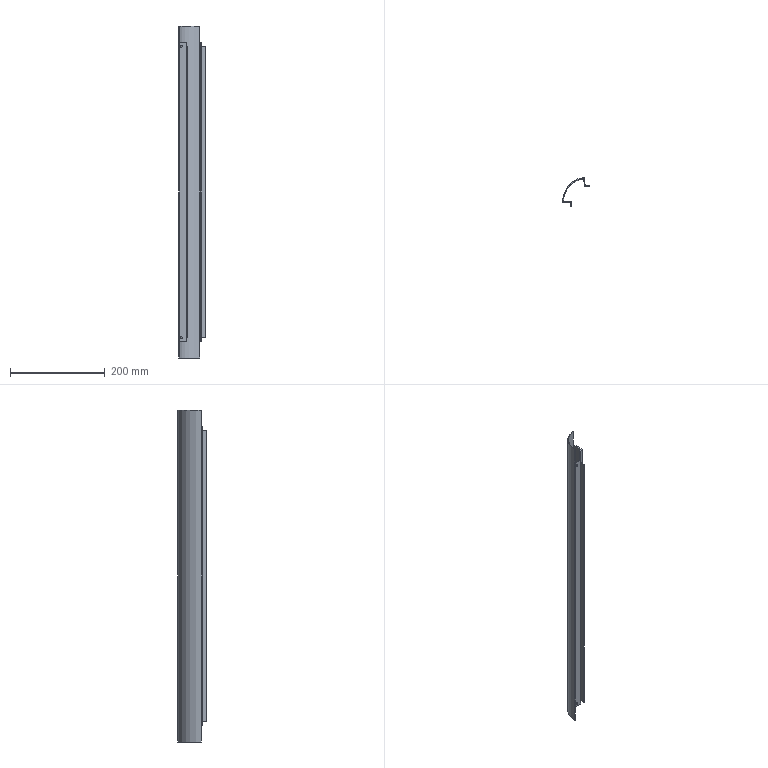Part | SolidWorks | features EdgeFlange 4, ICE 2, FlatPattern 1, SMBaseFlange 1, SheetMetal 1 | 1 solid | 51 faces | box 56.016 x 59.625 x 700 mm | volume 123971 mm3 | plane 36 | cylinder 15 | commonest cylinder face diameters 3 x5 4.5 x4 6.5 x4 97 x1 100 x1
STEP:
#1=CARTESIAN_POINT('',(-4.744,37.955,-175.));
#2=VERTEX_POINT('',#1);
#3=CARTESIAN_POINT('',(-5.551,44.404,-175.));
#4=VERTEX_POINT('',#3);
#5=CARTESIAN_POINT('',(-5.147,41.18,-175.));
#6=DIRECTION('',(0.9923,0.124,0.));
#7=DIRECTION('',(-0.124,0.9923,0.));
#8=AXIS2_PLACEMENT_3D('',#5,#6,#7);
#9=CIRCLE('',#8,3.25);
#10=EDGE_CURVE('',#2,#4,#9,.T.);
#11=ORIENTED_EDGE('',*,*,#10,.F.);
#12=CARTESIAN_POINT('',(-3.256,38.141,-175.));
#13=VERTEX_POINT('',#12);
#14=CARTESIAN_POINT('',(-4.744,37.955,-175.));
#15=DIRECTION('',(0.9923,0.124,0.));
#16=VECTOR('',#15,1000.);
#17=LINE('',#14,#16);
#18=EDGE_CURVE('',#2,#13,#17,.T.);
#19=ORIENTED_EDGE('',*,*,#18,.T.);
#20=CARTESIAN_POINT('',(-4.062,44.59,-175.));
#21=VERTEX_POINT('',#20);
#22=CARTESIAN_POINT('',(-3.659,41.366,-175.));
#23=DIRECTION('',(0.9923,0.124,0.));
#24=DIRECTION('',(-0.124,0.9923,0.));
#25=AXIS2_PLACEMENT_3D('',#22,#23,#24);
#26=CIRCLE('',#25,3.25);
#27=EDGE_CURVE('',#13,#21,#26,.T.);
#28=ORIENTED_EDGE('',*,*,#27,.T.);
#29=CARTESIAN_POINT('',(-5.551,44.404,-175.));
#30=DIRECTION('',(0.9923,0.124,0.));
#31=VECTOR('',#30,1000.);
#32=LINE('',#29,#31);
#33=EDGE_CURVE('',#4,#21,#32,.T.);
#34=ORIENTED_EDGE('',*,*,#33,.F.);
#35=EDGE_LOOP('',(#11,#19,#28,#34));
#36=FACE_OUTER_BOUND('',#35,.T.);
#37=CARTESIAN_POINT('',(-5.147,41.18,-175.));
#38=DIRECTION('',(0.9923,0.124,0.));
#39=DIRECTION('',(-0.124,0.9923,0.));
#40=AXIS2_PLACEMENT_3D('',#37,#38,#39);
#41=CYLINDRICAL_SURFACE('',#40,3.25);
#42=ADVANCED_FACE('',(#36),#41,.F.);
#43=CARTESIAN_POINT('',(-4.744,37.955,175.));
#44=VERTEX_POINT('',#43);
#45=CARTESIAN_POINT('',(-5.551,44.404,175.));
#46=VERTEX_POINT('',#45);
#47=CARTESIAN_POINT('',(-5.147,41.18,175.));
#48=DIRECTION('',(0.9923,0.124,0.));
#49=DIRECTION('',(-0.124,0.9923,0.));
#50=AXIS2_PLACEMENT_3D('',#47,#48,#49);
#51=CIRCLE('',#50,3.25);
#52=EDGE_CURVE('',#44,#46,#51,.T.);
#53=ORIENTED_EDGE('',*,*,#52,.F.);
#54=CARTESIAN_POINT('',(-3.256,38.141,175.));
#55=VERTEX_POINT('',#54);
#56=CARTESIAN_POINT('',(-4.744,37.955,175.));
#57=DIRECTION('',(0.9923,0.124,0.));
#58=VECTOR('',#57,1000.);
#59=LINE('',#56,#58);
#60=EDGE_CURVE('',#44,#55,#59,.T.);
#61=ORIENTED_EDGE('',*,*,#60,.T.);
#62=CARTESIAN_POINT('',(-4.062,44.59,175.));
#63=VERTEX_POINT('',#62);
#64=CARTESIAN_POINT('',(-3.659,41.366,175.));
#65=DIRECTION('',(0.9923,0.124,0.));
#66=DIRECTION('',(-0.124,0.9923,0.));
#67=AXIS2_PLACEMENT_3D('',#64,#65,#66);
#68=CIRCLE('',#67,3.25);
#69=EDGE_CURVE('',#55,#63,#68,.T.);
#70=ORIENTED_EDGE('',*,*,#69,.T.);
#71=CARTESIAN_POINT('',(-5.551,44.404,175.));
#72=DIRECTION('',(0.9923,0.124,0.));
#73=VECTOR('',#72,1000.);
#74=LINE('',#71,#73);
#75=EDGE_CURVE('',#46,#63,#74,.T.);
#76=ORIENTED_EDGE('',*,*,#75,.F.);
#77=EDGE_LOOP('',(#53,#61,#70,#76));
#78=FACE_OUTER_BOUND('',#77,.T.);
#79=CARTESIAN_POINT('',(-5.147,41.18,175.));
#80=DIRECTION('',(0.9923,0.124,0.));
#81=DIRECTION('',(-0.124,0.9923,0.));
#82=AXIS2_PLACEMENT_3D('',#79,#80,#81);
#83=CYLINDRICAL_SURFACE('',#82,3.25);
#84=ADVANCED_FACE('',(#78),#83,.F.);
#85=CARTESIAN_POINT('',(-46.75,0.,-307.5));
#86=VERTEX_POINT('',#85);
#87=CARTESIAN_POINT('',(-42.25,0.,-307.5));
#88=VERTEX_POINT('',#87);
#89=CARTESIAN_POINT('',(-44.5,0.,-307.5));
#90=DIRECTION('',(0.,-1.,0.));
#91=DIRECTION('',(1.,0.,0.));
#92=AXIS2_PLACEMENT_3D('',#89,#90,#91);
#93=CIRCLE('',#92,2.25);
#94=EDGE_CURVE('',#86,#88,#93,.T.);
#95=ORIENTED_EDGE('',*,*,#94,.F.);
#96=CARTESIAN_POINT('',(-46.75,-1.5,-307.5));
#97=VERTEX_POINT('',#96);
#98=CARTESIAN_POINT('',(-46.75,0.,-307.5));
#99=DIRECTION('',(0.,-1.,0.));
#100=VECTOR('',#99,1000.);
#101=LINE('',#98,#100);
#102=EDGE_CURVE('',#86,#97,#101,.T.);
#103=ORIENTED_EDGE('',*,*,#102,.T.);
#104=CARTESIAN_POINT('',(-42.25,-1.5,-307.5));
#105=VERTEX_POINT('',#104);
#106=CARTESIAN_POINT('',(-44.5,-1.5,-307.5));
#107=DIRECTION('',(0.,-1.,0.));
#108=DIRECTION('',(1.,0.,0.));
#109=AXIS2_PLACEMENT_3D('',#106,#107,#108);
#110=CIRCLE('',#109,2.25);
#111=EDGE_CURVE('',#97,#105,#110,.T.);
#112=ORIENTED_EDGE('',*,*,#111,.T.);
#113=CARTESIAN_POINT('',(-42.25,0.,-307.5));
#114=DIRECTION('',(0.,-1.,0.));
#115=VECTOR('',#114,1000.);
#116=LINE('',#113,#115);
#117=EDGE_CURVE('',#88,#105,#116,.T.);
#118=ORIENTED_EDGE('',*,*,#117,.F.);
#119=EDGE_LOOP('',(#95,#103,#112,#118));
#120=FACE_OUTER_BOUND('',#119,.T.);
#121=CARTESIAN_POINT('',(-44.5,0.,-307.5));
#122=DIRECTION('',(0.,-1.,0.));
#123=DIRECTION('',(1.,0.,0.));
#124=AXIS2_PLACEMENT_3D('',#121,#122,#123);
#125=CYLINDRICAL_SURFACE('',#124,2.25);
#126=ADVANCED_FACE('',(#120),#125,.F.);
#127=CARTESIAN_POINT('',(-46.75,0.,307.5));
#128=VERTEX_POINT('',#127);
#129=CARTESIAN_POINT('',(-42.25,0.,307.5));
#130=VERTEX_POINT('',#129);
#131=CARTESIAN_POINT('',(-44.5,0.,307.5));
#132=DIRECTION('',(0.,-1.,0.));
#133=DIRECTION('',(1.,0.,0.));
#134=AXIS2_PLACEMENT_3D('',#131,#132,#133);
#135=CIRCLE('',#134,2.25);
#136=EDGE_CURVE('',#128,#130,#135,.T.);
#137=ORIENTED_EDGE('',*,*,#136,.F.);
#138=CARTESIAN_POINT('',(-46.75,-1.5,307.5));
#139=VERTEX_POINT('',#138);
#140=CARTESIAN_POINT('',(-46.75,0.,307.5));
#141=DIRECTION('',(0.,-1.,0.));
#142=VECTOR('',#141,1000.);
#143=LINE('',#140,#142);
#144=EDGE_CURVE('',#128,#139,#143,.T.);
#145=ORIENTED_EDGE('',*,*,#144,.T.);
#146=CARTESIAN_POINT('',(-42.25,-1.5,307.5));
#147=VERTEX_POINT('',#146);
#148=CARTESIAN_POINT('',(-44.5,-1.5,307.5));
#149=DIRECTION('',(0.,-1.,0.));
#150=DIRECTION('',(1.,0.,0.));
#151=AXIS2_PLACEMENT_3D('',#148,#149,#150);
#152=CIRCLE('',#151,2.25);
#153=EDGE_CURVE('',#139,#147,#152,.T.);
#154=ORIENTED_EDGE('',*,*,#153,.T.);
#155=CARTESIAN_POINT('',(-42.25,0.,307.5));
#156=DIRECTION('',(0.,-1.,0.));
#157=VECTOR('',#156,1000.);
#158=LINE('',#155,#157);
#159=EDGE_CURVE('',#130,#147,#158,.T.);
#160=ORIENTED_EDGE('',*,*,#159,.F.);
#161=EDGE_LOOP('',(#137,#145,#154,#160));
#162=FACE_OUTER_BOUND('',#161,.T.);
#163=CARTESIAN_POINT('',(-44.5,0.,307.5));
#164=DIRECTION('',(0.,-1.,0.));
#165=DIRECTION('',(1.,0.,0.));
#166=AXIS2_PLACEMENT_3D('',#163,#164,#165);
#167=CYLINDRICAL_SURFACE('',#166,2.25);
#168=ADVANCED_FACE('',(#162),#167,.F.);
#169=CARTESIAN_POINT('',(-6.202,49.614,315.));
#170=VERTEX_POINT('',#169);
#171=CARTESIAN_POINT('',(-6.016,49.625,315.));
#172=VERTEX_POINT('',#171);
#173=CARTESIAN_POINT('',(-6.016,48.125,315.));
#174=DIRECTION('',(0.,0.,-1.));
#175=DIRECTION('',(0.,1.,0.));
#176=AXIS2_PLACEMENT_3D('',#173,#174,#175);
#177=CIRCLE('',#176,1.5);
#178=EDGE_CURVE('',#170,#172,#177,.T.);
#179=ORIENTED_EDGE('',*,*,#178,.T.);
#180=CARTESIAN_POINT('',(-6.016,49.625,-315.));
#181=VERTEX_POINT('',#180);
#182=CARTESIAN_POINT('',(-6.016,49.625,-315.));
#183=DIRECTION('',(0.,0.,-1.));
#184=VECTOR('',#183,1000.);
#185=LINE('',#182,#184);
#186=EDGE_CURVE('',#172,#181,#185,.T.);
#187=ORIENTED_EDGE('',*,*,#186,.T.);
#188=CARTESIAN_POINT('',(-6.202,49.614,-315.));
#189=VERTEX_POINT('',#188);
#190=CARTESIAN_POINT('',(-6.016,48.125,-315.));
#191=DIRECTION('',(0.,0.,-1.));
#192=DIRECTION('',(0.,1.,0.));
#193=AXIS2_PLACEMENT_3D('',#190,#191,#192);
#194=CIRCLE('',#193,1.5);
#195=EDGE_CURVE('',#189,#181,#194,.T.);
#196=ORIENTED_EDGE('',*,*,#195,.F.);
#197=CARTESIAN_POINT('',(-6.202,49.614,-315.));
#198=DIRECTION('',(0.,0.,-1.));
#199=VECTOR('',#198,1000.);
#200=LINE('',#197,#199);
#201=EDGE_CURVE('',#170,#189,#200,.T.);
#202=ORIENTED_EDGE('',*,*,#201,.F.);
#203=EDGE_LOOP('',(#179,#187,#196,#202));
#204=FACE_OUTER_BOUND('',#203,.T.);
#205=CARTESIAN_POINT('',(-6.016,48.125,-315.));
#206=DIRECTION('',(0.,0.,-1.));
#207=DIRECTION('',(0.,1.,0.));
#208=AXIS2_PLACEMENT_3D('',#205,#206,#207);
#209=CYLINDRICAL_SURFACE('',#208,1.5);
#210=ADVANCED_FACE('',(#204),#209,.T.);
#211=CARTESIAN_POINT('',(-33.,0.,306.5));
#212=VERTEX_POINT('',#211);
#213=CARTESIAN_POINT('',(-33.,-1.5,306.5));
#214=VERTEX_POINT('',#213);
#215=CARTESIAN_POINT('',(-33.,0.,306.5));
#216=DIRECTION('',(0.,-1.,0.));
#217=VECTOR('',#216,1000.);
#218=LINE('',#215,#217);
#219=EDGE_CURVE('',#212,#214,#218,.T.);
#220=ORIENTED_EDGE('',*,*,#219,.F.);
#221=CARTESIAN_POINT('',(-33.,0.,315.));
#222=VERTEX_POINT('',#221);
#223=CARTESIAN_POINT('',(-33.,0.,315.));
#224=DIRECTION('',(0.,0.,1.));
#225=VECTOR('',#224,1000.);
#226=LINE('',#223,#225);
#227=EDGE_CURVE('',#212,#222,#226,.T.);
#228=ORIENTED_EDGE('',*,*,#227,.T.);
#229=CARTESIAN_POINT('',(-33.,-1.5,315.));
#230=VERTEX_POINT('',#229);
#231=CARTESIAN_POINT('',(-33.,-1.5,315.));
#232=DIRECTION('',(0.,1.,0.));
#233=VECTOR('',#232,1000.);
#234=LINE('',#231,#233);
#235=EDGE_CURVE('',#230,#222,#234,.T.);
#236=ORIENTED_EDGE('',*,*,#235,.F.);
#237=CARTESIAN_POINT('',(-33.,-1.5,315.));
#238=DIRECTION('',(0.,0.,1.));
#239=VECTOR('',#238,1000.);
#240=LINE('',#237,#239);
#241=EDGE_CURVE('',#214,#230,#240,.T.);
#242=ORIENTED_EDGE('',*,*,#241,.F.);
#243=EDGE_LOOP('',(#220,#228,#236,#242));
#244=FACE_OUTER_BOUND('',#243,.T.);
#245=CARTESIAN_POINT('',(-33.,-1.5,315.));
#246=DIRECTION('',(-1.,0.,0.));
#247=DIRECTION('',(0.,-1.,0.));
#248=AXIS2_PLACEMENT_3D('',#245,#246,#247);
#249=PLANE('',#248);
#250=ADVANCED_FACE('',(#244),#249,.F.);
#251=CARTESIAN_POINT('',(-50.,0.,350.));
#252=VERTEX_POINT('',#251);
#253=CARTESIAN_POINT('',(-50.,0.,315.));
#254=VERTEX_POINT('',#253);
#255=CARTESIAN_POINT('',(-50.,0.,350.));
#256=DIRECTION('',(0.,0.,-1.));
#257=VECTOR('',#256,1000.);
#258=LINE('',#255,#257);
#259=EDGE_CURVE('',#252,#254,#258,.T.);
#260=ORIENTED_EDGE('',*,*,#259,.T.);
#261=CARTESIAN_POINT('',(-48.5,0.,315.));
#262=VERTEX_POINT('',#261);
#263=CARTESIAN_POINT('',(-50.,0.,315.));
#264=DIRECTION('',(1.,0.,0.));
#265=VECTOR('',#264,1000.);
#266=LINE('',#263,#265);
#267=EDGE_CURVE('',#254,#262,#266,.T.);
#268=ORIENTED_EDGE('',*,*,#267,.T.);
#269=CARTESIAN_POINT('',(-48.5,0.,350.));
#270=VERTEX_POINT('',#269);
#271=CARTESIAN_POINT('',(-48.5,0.,350.));
#272=DIRECTION('',(0.,0.,-1.));
#273=VECTOR('',#272,1000.);
#274=LINE('',#271,#273);
#275=EDGE_CURVE('',#270,#262,#274,.T.);
#276=ORIENTED_EDGE('',*,*,#275,.F.);
#277=CARTESIAN_POINT('',(-48.5,0.,350.));
#278=DIRECTION('',(-1.,0.,0.));
#279=VECTOR('',#278,1000.);
#280=LINE('',#277,#279);
#281=EDGE_CURVE('',#270,#252,#280,.T.);
#282=ORIENTED_EDGE('',*,*,#281,.T.);
#283=EDGE_LOOP('',(#260,#268,#276,#282));
#284=FACE_OUTER_BOUND('',#283,.T.);
#285=CARTESIAN_POINT('',(-48.5,0.,350.));
#286=DIRECTION('',(0.,-1.,0.));
#287=DIRECTION('',(1.,0.,0.));
#288=AXIS2_PLACEMENT_3D('',#285,#286,#287);
#289=PLANE('',#288);
#290=ADVANCED_FACE('',(#284),#289,.T.);
#291=CARTESIAN_POINT('',(-4.093,32.745,306.5));
#292=VERTEX_POINT('',#291);
#293=CARTESIAN_POINT('',(-4.093,32.745,315.));
#294=VERTEX_POINT('',#293);
#295=CARTESIAN_POINT('',(-4.093,32.745,315.));
#296=DIRECTION('',(0.,0.,1.));
#297=VECTOR('',#296,1000.);
#298=LINE('',#295,#297);
#299=EDGE_CURVE('',#292,#294,#298,.T.);
#300=ORIENTED_EDGE('',*,*,#299,.F.);
#301=CARTESIAN_POINT('',(-2.605,32.931,306.5));
#302=VERTEX_POINT('',#301);
#303=CARTESIAN_POINT('',(-4.093,32.745,306.5));
#304=DIRECTION('',(0.9923,0.124,0.));
#305=VECTOR('',#304,1000.);
#306=LINE('',#303,#305);
#307=EDGE_CURVE('',#292,#302,#306,.T.);
#308=ORIENTED_EDGE('',*,*,#307,.T.);
#309=CARTESIAN_POINT('',(-2.605,32.931,315.));
#310=VERTEX_POINT('',#309);
#311=CARTESIAN_POINT('',(-2.605,32.931,315.));
#312=DIRECTION('',(0.,0.,1.));
#313=VECTOR('',#312,1000.);
#314=LINE('',#311,#313);
#315=EDGE_CURVE('',#302,#310,#314,.T.);
#316=ORIENTED_EDGE('',*,*,#315,.T.);
#317=CARTESIAN_POINT('',(-2.605,32.931,315.));
#318=DIRECTION('',(-0.9923,-0.124,0.));
#319=VECTOR('',#318,1000.);
#320=LINE('',#317,#319);
#321=EDGE_CURVE('',#310,#294,#320,.T.);
#322=ORIENTED_EDGE('',*,*,#321,.T.);
#323=EDGE_LOOP('',(#300,#308,#316,#322));
#324=FACE_OUTER_BOUND('',#323,.T.);
#325=CARTESIAN_POINT('',(-2.605,32.931,315.));
#326=DIRECTION('',(0.124,-0.9923,0.));
#327=DIRECTION('',(0.9923,0.124,0.));
#328=AXIS2_PLACEMENT_3D('',#325,#326,#327);
#329=PLANE('',#328);
#330=ADVANCED_FACE('',(#324),#329,.T.);
#331=CARTESIAN_POINT('',(-6.202,49.614,-350.));
#332=VERTEX_POINT('',#331);
#333=CARTESIAN_POINT('',(-6.202,49.614,350.));
#334=DIRECTION('',(0.,0.,-1.));
#335=VECTOR('',#334,1000.);
#336=LINE('',#333,#335);
#337=EDGE_CURVE('',#189,#332,#336,.T.);
#338=ORIENTED_EDGE('',*,*,#337,.F.);
#339=CARTESIAN_POINT('',(-6.016,48.125,-315.));
#340=VERTEX_POINT('',#339);
#341=CARTESIAN_POINT('',(-6.202,49.614,-315.));
#342=DIRECTION('',(0.124,-0.9923,0.));
#343=VECTOR('',#342,1000.);
#344=LINE('',#341,#343);
#345=EDGE_CURVE('',#189,#340,#344,.T.);
#346=ORIENTED_EDGE('',*,*,#345,.T.);
#347=CARTESIAN_POINT('',(-6.016,48.125,-350.));
#348=VERTEX_POINT('',#347);
#349=CARTESIAN_POINT('',(-6.016,48.125,350.));
#350=DIRECTION('',(0.,0.,-1.));
#351=VECTOR('',#350,1000.);
#352=LINE('',#349,#351);
#353=EDGE_CURVE('',#340,#348,#352,.T.);
#354=ORIENTED_EDGE('',*,*,#353,.T.);
#355=CARTESIAN_POINT('',(-6.202,49.614,-350.));
#356=DIRECTION('',(0.124,-0.9923,0.));
#357=VECTOR('',#356,1000.);
#358=LINE('',#355,#357);
#359=EDGE_CURVE('',#332,#348,#358,.T.);
#360=ORIENTED_EDGE('',*,*,#359,.F.);
#361=EDGE_LOOP('',(#338,#346,#354,#360));
#362=FACE_OUTER_BOUND('',#361,.T.);
#363=CARTESIAN_POINT('',(-6.202,49.614,350.));
#364=DIRECTION('',(0.9923,0.124,0.));
#365=DIRECTION('',(-0.124,0.9923,0.));
#366=AXIS2_PLACEMENT_3D('',#363,#364,#365);
#367=PLANE('',#366);
#368=ADVANCED_FACE('',(#362),#367,.T.);
#369=CARTESIAN_POINT('',(-50.,0.,-350.));
#370=VERTEX_POINT('',#369);
#371=CARTESIAN_POINT('',(0.,0.,-350.));
#372=DIRECTION('',(0.,0.,1.));
#373=DIRECTION('',(1.,0.,0.));
#374=AXIS2_PLACEMENT_3D('',#371,#372,#373);
#375=CIRCLE('',#374,50.);
#376=EDGE_CURVE('',#332,#370,#375,.T.);
#377=ORIENTED_EDGE('',*,*,#376,.T.);
#378=CARTESIAN_POINT('',(-50.,0.,-315.));
#379=VERTEX_POINT('',#378);
#380=CARTESIAN_POINT('',(-50.,0.,350.));
#381=DIRECTION('',(0.,0.,-1.));
#382=VECTOR('',#381,1000.);
#383=LINE('',#380,#382);
#384=EDGE_CURVE('',#379,#370,#383,.T.);
#385=ORIENTED_EDGE('',*,*,#384,.F.);
#386=CARTESIAN_POINT('',(-50.,0.,315.));
#387=DIRECTION('',(0.,0.,-1.));
#388=VECTOR('',#387,1000.);
#389=LINE('',#386,#388);
#390=EDGE_CURVE('',#254,#379,#389,.T.);
#391=ORIENTED_EDGE('',*,*,#390,.F.);
#392=ORIENTED_EDGE('',*,*,#259,.F.);
#393=CARTESIAN_POINT('',(-6.202,49.614,350.));
#394=VERTEX_POINT('',#393);
#395=CARTESIAN_POINT('',(0.,0.,350.));
#396=DIRECTION('',(0.,0.,1.));
#397=DIRECTION('',(1.,0.,0.));
#398=AXIS2_PLACEMENT_3D('',#395,#396,#397);
#399=CIRCLE('',#398,50.);
#400=EDGE_CURVE('',#394,#252,#399,.T.);
#401=ORIENTED_EDGE('',*,*,#400,.F.);
#402=CARTESIAN_POINT('',(-6.202,49.614,350.));
#403=DIRECTION('',(0.,0.,-1.));
#404=VECTOR('',#403,1000.);
#405=LINE('',#402,#404);
#406=EDGE_CURVE('',#394,#170,#405,.T.);
#407=ORIENTED_EDGE('',*,*,#406,.T.);
#408=ORIENTED_EDGE('',*,*,#201,.T.);
#409=ORIENTED_EDGE('',*,*,#337,.T.);
#410=EDGE_LOOP('',(#377,#385,#391,#392,#401,#407,#408,#409));
#411=FACE_OUTER_BOUND('',#410,.T.);
#412=CARTESIAN_POINT('',(0.,0.,350.));
#413=DIRECTION('',(0.,0.,-1.));
#414=DIRECTION('',(-1.,0.,0.));
#415=AXIS2_PLACEMENT_3D('',#412,#413,#414);
#416=CYLINDRICAL_SURFACE('',#415,50.);
#417=ADVANCED_FACE('',(#411),#416,.T.);
#418=CARTESIAN_POINT('',(-48.5,0.,-315.));
#419=VERTEX_POINT('',#418);
#420=CARTESIAN_POINT('',(-50.,0.,-315.));
#421=DIRECTION('',(1.,0.,0.));
#422=VECTOR('',#421,1000.);
#423=LINE('',#420,#422);
#424=EDGE_CURVE('',#379,#419,#423,.T.);
#425=ORIENTED_EDGE('',*,*,#424,.F.);
#426=ORIENTED_EDGE('',*,*,#384,.T.);
#427=CARTESIAN_POINT('',(-48.5,0.,-350.));
#428=VERTEX_POINT('',#427);
#429=CARTESIAN_POINT('',(-48.5,0.,-350.));
#430=DIRECTION('',(-1.,0.,0.));
#431=VECTOR('',#430,1000.);
#432=LINE('',#429,#431);
#433=EDGE_CURVE('',#428,#370,#432,.T.);
#434=ORIENTED_EDGE('',*,*,#433,.F.);
#435=CARTESIAN_POINT('',(-48.5,0.,350.));
#436=DIRECTION('',(0.,0.,-1.));
#437=VECTOR('',#436,1000.);
#438=LINE('',#435,#437);
#439=EDGE_CURVE('',#419,#428,#438,.T.);
#440=ORIENTED_EDGE('',*,*,#439,.F.);
#441=EDGE_LOOP('',(#425,#426,#434,#440));
#442=FACE_OUTER_BOUND('',#441,.T.);
#443=CARTESIAN_POINT('',(-48.5,0.,350.));
#444=DIRECTION('',(0.,-1.,0.));
#445=DIRECTION('',(1.,0.,0.));
#446=AXIS2_PLACEMENT_3D('',#443,#444,#445);
#447=PLANE('',#446);
#448=ADVANCED_FACE('',(#442),#447,.T.);
#449=CARTESIAN_POINT('',(0.,0.,-350.));
#450=DIRECTION('',(0.,0.,1.));
#451=DIRECTION('',(1.,0.,0.));
#452=AXIS2_PLACEMENT_3D('',#449,#450,#451);
#453=CIRCLE('',#452,48.5);
#454=EDGE_CURVE('',#348,#428,#453,.T.);
#455=ORIENTED_EDGE('',*,*,#454,.F.);
#456=ORIENTED_EDGE('',*,*,#353,.F.);
#457=CARTESIAN_POINT('',(-6.016,48.125,315.));
#458=VERTEX_POINT('',#457);
#459=CARTESIAN_POINT('',(-6.016,48.125,-315.));
#460=DIRECTION('',(0.,0.,-1.));
#461=VECTOR('',#460,1000.);
#462=LINE('',#459,#461);
#463=EDGE_CURVE('',#458,#340,#462,.T.);
#464=ORIENTED_EDGE('',*,*,#463,.F.);
#465=CARTESIAN_POINT('',(-6.016,48.125,350.));
#466=VERTEX_POINT('',#465);
#467=CARTESIAN_POINT('',(-6.016,48.125,350.));
#468=DIRECTION('',(0.,0.,-1.));
#469=VECTOR('',#468,1000.);
#470=LINE('',#467,#469);
#471=EDGE_CURVE('',#466,#458,#470,.T.);
#472=ORIENTED_EDGE('',*,*,#471,.F.);
#473=CARTESIAN_POINT('',(0.,0.,350.));
#474=DIRECTION('',(0.,0.,1.));
#475=DIRECTION('',(1.,0.,0.));
#476=AXIS2_PLACEMENT_3D('',#473,#474,#475);
#477=CIRCLE('',#476,48.5);
#478=EDGE_CURVE('',#466,#270,#477,.T.);
#479=ORIENTED_EDGE('',*,*,#478,.T.);
#480=ORIENTED_EDGE('',*,*,#275,.T.);
#481=CARTESIAN_POINT('',(-48.5,0.,315.));
#482=DIRECTION('',(0.,0.,-1.));
#483=VECTOR('',#482,1000.);
#484=LINE('',#481,#483);
#485=EDGE_CURVE('',#262,#419,#484,.T.);
#486=ORIENTED_EDGE('',*,*,#485,.T.);
#487=ORIENTED_EDGE('',*,*,#439,.T.);
#488=EDGE_LOOP('',(#455,#456,#464,#472,#479,#480,#486,#487));
#489=FACE_OUTER_BOUND('',#488,.T.);
#490=CARTESIAN_POINT('',(0.,0.,350.));
#491=DIRECTION('',(0.,0.,-1.));
#492=DIRECTION('',(-1.,0.,0.));
#493=AXIS2_PLACEMENT_3D('',#490,#491,#492);
#494=CYLINDRICAL_SURFACE('',#493,48.5);
#495=ADVANCED_FACE('',(#489),#494,.F.);
#496=CARTESIAN_POINT('',(-6.202,49.614,315.));
#497=DIRECTION('',(0.124,-0.9923,0.));
#498=VECTOR('',#497,1000.);
#499=LINE('',#496,#498);
#500=EDGE_CURVE('',#170,#458,#499,.T.);
#501=ORIENTED_EDGE('',*,*,#500,.F.);
#502=ORIENTED_EDGE('',*,*,#406,.F.);
#503=CARTESIAN_POINT('',(-6.202,49.614,350.));
#504=DIRECTION('',(0.124,-0.9923,0.));
#505=VECTOR('',#504,1000.);
#506=LINE('',#503,#505);
#507=EDGE_CURVE('',#394,#466,#506,.T.);
#508=ORIENTED_EDGE('',*,*,#507,.T.);
#509=ORIENTED_EDGE('',*,*,#471,.T.);
#510=EDGE_LOOP('',(#501,#502,#508,#509));
#511=FACE_OUTER_BOUND('',#510,.T.);
#512=CARTESIAN_POINT('',(-6.202,49.614,350.));
#513=DIRECTION('',(0.9923,0.124,0.));
#514=DIRECTION('',(-0.124,0.9923,0.));
#515=AXIS2_PLACEMENT_3D('',#512,#513,#514);
#516=PLANE('',#515);
#517=ADVANCED_FACE('',(#511),#516,.T.);
#518=ORIENTED_EDGE('',*,*,#400,.T.);
#519=ORIENTED_EDGE('',*,*,#281,.F.);
#520=ORIENTED_EDGE('',*,*,#478,.F.);
#521=ORIENTED_EDGE('',*,*,#507,.F.);
#522=EDGE_LOOP('',(#518,#519,#520,#521));
#523=FACE_OUTER_BOUND('',#522,.T.);
#524=CARTESIAN_POINT('',(0.,0.,350.));
#525=DIRECTION('',(0.,0.,1.));
#526=DIRECTION('',(1.,0.,0.));
#527=AXIS2_PLACEMENT_3D('',#524,#525,#526);
#528=PLANE('',#527);
#529=ADVANCED_FACE('',(#523),#528,.T.);
#530=ORIENTED_EDGE('',*,*,#376,.F.);
#531=ORIENTED_EDGE('',*,*,#359,.T.);
#532=ORIENTED_EDGE('',*,*,#454,.T.);
#533=ORIENTED_EDGE('',*,*,#433,.T.);
#534=EDGE_LOOP('',(#530,#531,#532,#533));
#535=FACE_OUTER_BOUND('',#534,.T.);
#536=CARTESIAN_POINT('',(0.,0.,-350.));
#537=DIRECTION('',(0.,0.,1.));
#538=DIRECTION('',(1.,0.,0.));
#539=AXIS2_PLACEMENT_3D('',#536,#537,#538);
#540=PLANE('',#539);
#541=ADVANCED_FACE('',(#535),#540,.F.);
#542=ORIENTED_EDGE('',*,*,#178,.F.);
#543=ORIENTED_EDGE('',*,*,#500,.T.);
#544=CARTESIAN_POINT('',(-4.527,48.312,315.));
#545=VERTEX_POINT('',#544);
#546=CARTESIAN_POINT('',(-4.527,48.312,315.));
#547=DIRECTION('',(-0.9923,-0.124,0.));
#548=VECTOR('',#547,1000.);
#549=LINE('',#546,#548);
#550=EDGE_CURVE('',#545,#458,#549,.T.);
#551=ORIENTED_EDGE('',*,*,#550,.F.);
#552=CARTESIAN_POINT('',(-6.016,48.125,315.));
#553=DIRECTION('',(0.,0.,-1.));
#554=DIRECTION('',(0.,1.,0.));
#555=AXIS2_PLACEMENT_3D('',#552,#553,#554);
#556=CIRCLE('',#555,1.5);
#557=EDGE_CURVE('',#172,#545,#556,.T.);
#558=ORIENTED_EDGE('',*,*,#557,.F.);
#559=EDGE_LOOP('',(#542,#543,#551,#558));
#560=FACE_OUTER_BOUND('',#559,.T.);
#561=CARTESIAN_POINT('',(-6.202,49.614,315.));
#562=DIRECTION('',(0.,0.,1.));
#563=DIRECTION('',(0.,-1.,0.));
#564=AXIS2_PLACEMENT_3D('',#561,#562,#563);
#565=PLANE('',#564);
#566=ADVANCED_FACE('',(#560),#565,.T.);
#567=ORIENTED_EDGE('',*,*,#186,.F.);
#568=ORIENTED_EDGE('',*,*,#557,.T.);
#569=CARTESIAN_POINT('',(-4.527,48.312,-315.));
#570=VERTEX_POINT('',#569);
#571=CARTESIAN_POINT('',(-4.527,48.312,-315.));
#572=DIRECTION('',(0.,0.,-1.));
#573=VECTOR('',#572,1000.);
#574=LINE('',#571,#573);
#575=EDGE_CURVE('',#545,#570,#574,.T.);
#576=ORIENTED_EDGE('',*,*,#575,.T.);
#577=CARTESIAN_POINT('',(-6.016,48.125,-315.));
#578=DIRECTION('',(0.,0.,-1.));
#579=DIRECTION('',(0.,1.,0.));
#580=AXIS2_PLACEMENT_3D('',#577,#578,#579);
#581=CIRCLE('',#580,1.5);
#582=EDGE_CURVE('',#181,#570,#581,.T.);
#583=ORIENTED_EDGE('',*,*,#582,.F.);
#584=EDGE_LOOP('',(#567,#568,#576,#583));
#585=FACE_OUTER_BOUND('',#584,.T.);
#586=CARTESIAN_POINT('',(-6.016,48.125,-315.));
#587=DIRECTION('',(0.,0.,-1.));
#588=DIRECTION('',(0.,1.,0.));
#589=AXIS2_PLACEMENT_3D('',#586,#587,#588);
#590=CYLINDRICAL_SURFACE('',#589,1.5);
#591=ADVANCED_FACE('',(#585),#590,.T.);
#592=ORIENTED_EDGE('',*,*,#345,.F.);
#593=ORIENTED_EDGE('',*,*,#195,.T.);
#594=ORIENTED_EDGE('',*,*,#582,.T.);
#595=CARTESIAN_POINT('',(-4.527,48.312,-315.));
#596=DIRECTION('',(-0.9923,-0.124,0.));
#597=VECTOR('',#596,1000.);
#598=LINE('',#595,#597);
#599=EDGE_CURVE('',#570,#340,#598,.T.);
#600=ORIENTED_EDGE('',*,*,#599,.T.);
#601=EDGE_LOOP('',(#592,#593,#594,#600));
#602=FACE_OUTER_BOUND('',#601,.T.);
#603=CARTESIAN_POINT('',(-6.202,49.614,-315.));
#604=DIRECTION('',(0.,0.,1.));
#605=DIRECTION('',(0.,-1.,0.));
#606=AXIS2_PLACEMENT_3D('',#603,#604,#605);
#607=PLANE('',#606);
#608=ADVANCED_FACE('',(#602),#607,.F.);
#609=CARTESIAN_POINT('',(-6.016,48.125,315.));
#610=DIRECTION('',(-0.124,0.9923,0.));
#611=VECTOR('',#610,1000.);
#612=LINE('',#609,#611);
#613=EDGE_CURVE('',#294,#458,#612,.T.);
#614=ORIENTED_EDGE('',*,*,#613,.F.);
#615=ORIENTED_EDGE('',*,*,#321,.F.);
#616=CARTESIAN_POINT('',(-4.527,48.312,315.));
#617=DIRECTION('',(-0.124,0.9923,0.));
#618=VECTOR('',#617,1000.);
#619=LINE('',#616,#618);
#620=EDGE_CURVE('',#310,#545,#619,.T.);
#621=ORIENTED_EDGE('',*,*,#620,.T.);
#622=ORIENTED_EDGE('',*,*,#550,.T.);
#623=EDGE_LOOP('',(#614,#615,#621,#622));
#624=FACE_OUTER_BOUND('',#623,.T.);
#625=CARTESIAN_POINT('',(-4.527,48.312,315.));
#626=DIRECTION('',(0.,0.,1.));
#627=DIRECTION('',(1.,0.,0.));
#628=AXIS2_PLACEMENT_3D('',#625,#626,#627);
#629=PLANE('',#628);
#630=ADVANCED_FACE('',(#624),#629,.T.);
#631=CARTESIAN_POINT('',(-4.093,32.745,-306.5));
#632=VERTEX_POINT('',#631);
#633=CARTESIAN_POINT('',(-2.605,32.931,-306.5));
#634=VERTEX_POINT('',#633);
#635=CARTESIAN_POINT('',(-4.093,32.745,-306.5));
#636=DIRECTION('',(0.9923,0.124,0.));
#637=VECTOR('',#636,1000.);
#638=LINE('',#635,#637);
#639=EDGE_CURVE('',#632,#634,#638,.T.);
#640=ORIENTED_EDGE('',*,*,#639,.F.);
#641=CARTESIAN_POINT('',(-4.093,32.745,-315.));
#642=VERTEX_POINT('',#641);
#643=CARTESIAN_POINT('',(-4.093,32.745,315.));
#644=DIRECTION('',(0.,0.,1.));
#645=VECTOR('',#644,1000.);
#646=LINE('',#643,#645);
#647=EDGE_CURVE('',#642,#632,#646,.T.);
#648=ORIENTED_EDGE('',*,*,#647,.F.);
#649=CARTESIAN_POINT('',(-2.605,32.931,-315.));
#650=VERTEX_POINT('',#649);
#651=CARTESIAN_POINT('',(-2.605,32.931,-315.));
#652=DIRECTION('',(-0.9923,-0.124,0.));
#653=VECTOR('',#652,1000.);
#654=LINE('',#651,#653);
#655=EDGE_CURVE('',#650,#642,#654,.T.);
#656=ORIENTED_EDGE('',*,*,#655,.F.);
#657=CARTESIAN_POINT('',(-2.605,32.931,315.));
#658=DIRECTION('',(0.,0.,1.));
#659=VECTOR('',#658,1000.);
#660=LINE('',#657,#659);
#661=EDGE_CURVE('',#650,#634,#660,.T.);
#662=ORIENTED_EDGE('',*,*,#661,.T.);
#663=EDGE_LOOP('',(#640,#648,#656,#662));
#664=FACE_OUTER_BOUND('',#663,.T.);
#665=CARTESIAN_POINT('',(-2.605,32.931,315.));
#666=DIRECTION('',(0.124,-0.9923,0.));
#667=DIRECTION('',(0.9923,0.124,0.));
#668=AXIS2_PLACEMENT_3D('',#665,#666,#667);
#669=PLANE('',#668);
#670=ADVANCED_FACE('',(#664),#669,.T.);
#671=CARTESIAN_POINT('',(-4.093,32.745,-315.));
#672=DIRECTION('',(0.124,-0.9923,0.));
#673=VECTOR('',#672,1000.);
#674=LINE('',#671,#673);
#675=EDGE_CURVE('',#340,#642,#674,.T.);
#676=ORIENTED_EDGE('',*,*,#675,.F.);
#677=ORIENTED_EDGE('',*,*,#599,.F.);
#678=CARTESIAN_POINT('',(-2.605,32.931,-315.));
#679=DIRECTION('',(0.124,-0.9923,0.));
#680=VECTOR('',#679,1000.);
#681=LINE('',#678,#680);
#682=EDGE_CURVE('',#570,#650,#681,.T.);
#683=ORIENTED_EDGE('',*,*,#682,.T.);
#684=ORIENTED_EDGE('',*,*,#655,.T.);
#685=EDGE_LOOP('',(#676,#677,#683,#684));
#686=FACE_OUTER_BOUND('',#685,.T.);
#687=CARTESIAN_POINT('',(-2.605,32.931,-315.));
#688=DIRECTION('',(0.,0.,-1.));
#689=DIRECTION('',(-1.,0.,0.));
#690=AXIS2_PLACEMENT_3D('',#687,#688,#689);
#691=PLANE('',#690);
#692=ADVANCED_FACE('',(#686),#691,.T.);
#693=CARTESIAN_POINT('',(-3.659,41.366,-175.));
#694=DIRECTION('',(0.9923,0.124,0.));
#695=DIRECTION('',(-0.124,0.9923,0.));
#696=AXIS2_PLACEMENT_3D('',#693,#694,#695);
#697=CIRCLE('',#696,3.25);
#698=EDGE_CURVE('',#21,#13,#697,.T.);
#699=ORIENTED_EDGE('',*,*,#698,.F.);
#700=ORIENTED_EDGE('',*,*,#27,.F.);
#701=EDGE_LOOP('',(#699,#700));
#702=FACE_BOUND('',#701,.T.);
#703=CARTESIAN_POINT('',(-3.659,41.366,175.));
#704=DIRECTION('',(0.9923,0.124,0.));
#705=DIRECTION('',(-0.124,0.9923,0.));
#706=AXIS2_PLACEMENT_3D('',#703,#704,#705);
#707=CIRCLE('',#706,3.25);
#708=EDGE_CURVE('',#63,#55,#707,.T.);
#709=ORIENTED_EDGE('',*,*,#708,.F.);
#710=ORIENTED_EDGE('',*,*,#69,.F.);
#711=EDGE_LOOP('',(#709,#710));
#712=FACE_BOUND('',#711,.T.);
#713=ORIENTED_EDGE('',*,*,#575,.F.);
#714=ORIENTED_EDGE('',*,*,#620,.F.);
#715=ORIENTED_EDGE('',*,*,#315,.F.);
#716=CARTESIAN_POINT('',(-2.605,32.931,-306.5));
#717=DIRECTION('',(0.,0.,-1.));
#718=VECTOR('',#717,1000.);
#719=LINE('',#716,#718);
#720=EDGE_CURVE('',#302,#634,#719,.T.);
#721=ORIENTED_EDGE('',*,*,#720,.T.);
#722=ORIENTED_EDGE('',*,*,#661,.F.);
#723=ORIENTED_EDGE('',*,*,#682,.F.);
#724=EDGE_LOOP('',(#713,#714,#715,#721,#722,#723));
#725=FACE_OUTER_BOUND('',#724,.T.);
#726=CARTESIAN_POINT('',(-4.527,48.312,315.));
#727=DIRECTION('',(0.9923,0.124,0.));
#728=DIRECTION('',(-0.124,0.9923,0.));
#729=AXIS2_PLACEMENT_3D('',#726,#727,#728);
#730=PLANE('',#729);
#731=ADVANCED_FACE('',(#702,#712,#725),#730,.T.);
#732=CARTESIAN_POINT('',(-5.147,41.18,-175.));
#733=DIRECTION('',(0.9923,0.124,0.));
#734=DIRECTION('',(-0.124,0.9923,0.));
#735=AXIS2_PLACEMENT_3D('',#732,#733,#734);
#736=CIRCLE('',#735,3.25);
#737=EDGE_CURVE('',#4,#2,#736,.T.);
#738=ORIENTED_EDGE('',*,*,#737,.T.);
#739=ORIENTED_EDGE('',*,*,#10,.T.);
#740=EDGE_LOOP('',(#738,#739));
#741=FACE_BOUND('',#740,.T.);
#742=CARTESIAN_POINT('',(-5.147,41.18,175.));
#743=DIRECTION('',(0.9923,0.124,0.));
#744=DIRECTION('',(-0.124,0.9923,0.));
#745=AXIS2_PLACEMENT_3D('',#742,#743,#744);
#746=CIRCLE('',#745,3.25);
#747=EDGE_CURVE('',#46,#44,#746,.T.);
#748=ORIENTED_EDGE('',*,*,#747,.T.);
#749=ORIENTED_EDGE('',*,*,#52,.T.);
#750=EDGE_LOOP('',(#748,#749));
#751=FACE_BOUND('',#750,.T.);
#752=ORIENTED_EDGE('',*,*,#463,.T.);
#753=ORIENTED_EDGE('',*,*,#675,.T.);
#754=ORIENTED_EDGE('',*,*,#647,.T.);
#755=CARTESIAN_POINT('',(-4.093,32.745,-306.5));
#756=DIRECTION('',(0.,0.,-1.));
#757=VECTOR('',#756,1000.);
#758=LINE('',#755,#757);
#759=EDGE_CURVE('',#292,#632,#758,.T.);
#760=ORIENTED_EDGE('',*,*,#759,.F.);
#761=ORIENTED_EDGE('',*,*,#299,.T.);
#762=ORIENTED_EDGE('',*,*,#613,.T.);
#763=EDGE_LOOP('',(#752,#753,#754,#760,#761,#762));
#764=FACE_OUTER_BOUND('',#763,.T.);
#765=CARTESIAN_POINT('',(-6.016,48.125,315.));
#766=DIRECTION('',(0.9923,0.124,0.));
#767=DIRECTION('',(-0.124,0.9923,0.));
#768=AXIS2_PLACEMENT_3D('',#765,#766,#767);
#769=PLANE('',#768);
#770=ADVANCED_FACE('',(#741,#751,#764),#769,.F.);
#771=CARTESIAN_POINT('',(-2.419,31.443,-306.5));
#772=VERTEX_POINT('',#771);
#773=CARTESIAN_POINT('',(-2.605,32.931,-306.5));
#774=DIRECTION('',(0.,0.,1.));
#775=DIRECTION('',(1.,0.,0.));
#776=AXIS2_PLACEMENT_3D('',#773,#774,#775);
#777=CIRCLE('',#776,1.5);
#778=EDGE_CURVE('',#632,#772,#777,.T.);
#779=ORIENTED_EDGE('',*,*,#778,.F.);
#780=ORIENTED_EDGE('',*,*,#639,.T.);
#781=CARTESIAN_POINT('',(-2.419,31.443,-306.5));
#782=DIRECTION('',(-0.124,0.9923,0.));
#783=VECTOR('',#782,1000.);
#784=LINE('',#781,#783);
#785=EDGE_CURVE('',#772,#634,#784,.T.);
#786=ORIENTED_EDGE('',*,*,#785,.F.);
#787=EDGE_LOOP('',(#779,#780,#786));
#788=FACE_OUTER_BOUND('',#787,.T.);
#789=CARTESIAN_POINT('',(-4.093,32.745,-306.5));
#790=DIRECTION('',(0.,0.,-1.));
#791=DIRECTION('',(-1.,0.,0.));
#792=AXIS2_PLACEMENT_3D('',#789,#790,#791);
#793=PLANE('',#792);
#794=ADVANCED_FACE('',(#788),#793,.T.);
#795=CARTESIAN_POINT('',(-2.419,31.443,306.5));
#796=VERTEX_POINT('',#795);
#797=CARTESIAN_POINT('',(-2.605,32.931,306.5));
#798=DIRECTION('',(0.,0.,1.));
#799=DIRECTION('',(1.,0.,0.));
#800=AXIS2_PLACEMENT_3D('',#797,#798,#799);
#801=CIRCLE('',#800,1.5);
#802=EDGE_CURVE('',#292,#796,#801,.T.);
#803=ORIENTED_EDGE('',*,*,#802,.F.);
#804=ORIENTED_EDGE('',*,*,#759,.T.);
#805=ORIENTED_EDGE('',*,*,#778,.T.);
#806=CARTESIAN_POINT('',(-2.419,31.443,-306.5));
#807=DIRECTION('',(0.,0.,-1.));
#808=VECTOR('',#807,1000.);
#809=LINE('',#806,#808);
#810=EDGE_CURVE('',#796,#772,#809,.T.);
#811=ORIENTED_EDGE('',*,*,#810,.F.);
#812=EDGE_LOOP('',(#803,#804,#805,#811));
#813=FACE_OUTER_BOUND('',#812,.T.);
#814=CARTESIAN_POINT('',(-2.605,32.931,306.5));
#815=DIRECTION('',(0.,0.,1.));
#816=DIRECTION('',(1.,0.,0.));
#817=AXIS2_PLACEMENT_3D('',#814,#815,#816);
#818=CYLINDRICAL_SURFACE('',#817,1.5);
#819=ADVANCED_FACE('',(#813),#818,.T.);
#820=ORIENTED_EDGE('',*,*,#307,.F.);
#821=ORIENTED_EDGE('',*,*,#802,.T.);
#822=CARTESIAN_POINT('',(-2.419,31.443,306.5));
#823=DIRECTION('',(-0.124,0.9923,0.));
#824=VECTOR('',#823,1000.);
#825=LINE('',#822,#824);
#826=EDGE_CURVE('',#796,#302,#825,.T.);
#827=ORIENTED_EDGE('',*,*,#826,.T.);
#828=EDGE_LOOP('',(#820,#821,#827));
#829=FACE_OUTER_BOUND('',#828,.T.);
#830=CARTESIAN_POINT('',(-4.093,32.745,306.5));
#831=DIRECTION('',(0.,0.,-1.));
#832=DIRECTION('',(-1.,0.,0.));
#833=AXIS2_PLACEMENT_3D('',#830,#831,#832);
#834=PLANE('',#833);
#835=ADVANCED_FACE('',(#829),#834,.F.);
#836=CARTESIAN_POINT('',(5.83,33.986,-306.5));
#837=VERTEX_POINT('',#836);
#838=CARTESIAN_POINT('',(5.83,33.986,-306.5));
#839=DIRECTION('',(0.9923,0.124,0.));
#840=VECTOR('',#839,1000.);
#841=LINE('',#838,#840);
#842=EDGE_CURVE('',#634,#837,#841,.T.);
#843=ORIENTED_EDGE('',*,*,#842,.T.);
#844=CARTESIAN_POINT('',(6.016,32.497,-306.5));
#845=VERTEX_POINT('',#844);
#846=CARTESIAN_POINT('',(6.016,32.497,-306.5));
#847=DIRECTION('',(-0.124,0.9923,0.));
#848=VECTOR('',#847,1000.);
#849=LINE('',#846,#848);
#850=EDGE_CURVE('',#845,#837,#849,.T.);
#851=ORIENTED_EDGE('',*,*,#850,.F.);
#852=CARTESIAN_POINT('',(6.016,32.497,-306.5));
#853=DIRECTION('',(0.9923,0.124,0.));
#854=VECTOR('',#853,1000.);
#855=LINE('',#852,#854);
#856=EDGE_CURVE('',#772,#845,#855,.T.);
#857=ORIENTED_EDGE('',*,*,#856,.F.);
#858=ORIENTED_EDGE('',*,*,#785,.T.);
#859=EDGE_LOOP('',(#843,#851,#857,#858));
#860=FACE_OUTER_BOUND('',#859,.T.);
#861=CARTESIAN_POINT('',(6.016,32.497,-306.5));
#862=DIRECTION('',(0.,0.,1.));
#863=DIRECTION('',(1.,0.,0.));
#864=AXIS2_PLACEMENT_3D('',#861,#862,#863);
#865=PLANE('',#864);
#866=ADVANCED_FACE('',(#860),#865,.F.);
#867=CARTESIAN_POINT('',(5.83,33.986,306.5));
#868=VERTEX_POINT('',#867);
#869=CARTESIAN_POINT('',(5.83,33.986,306.5));
#870=DIRECTION('',(0.,0.,1.));
#871=VECTOR('',#870,1000.);
#872=LINE('',#869,#871);
#873=EDGE_CURVE('',#837,#868,#872,.T.);
#874=ORIENTED_EDGE('',*,*,#873,.T.);
#875=CARTESIAN_POINT('',(6.016,32.497,306.5));
#876=VERTEX_POINT('',#875);
#877=CARTESIAN_POINT('',(6.016,32.497,306.5));
#878=DIRECTION('',(-0.124,0.9923,0.));
#879=VECTOR('',#878,1000.);
#880=LINE('',#877,#879);
#881=EDGE_CURVE('',#876,#868,#880,.T.);
#882=ORIENTED_EDGE('',*,*,#881,.F.);
#883=CARTESIAN_POINT('',(6.016,32.497,306.5));
#884=DIRECTION('',(0.,0.,1.));
#885=VECTOR('',#884,1000.);
#886=LINE('',#883,#885);
#887=EDGE_CURVE('',#845,#876,#886,.T.);
#888=ORIENTED_EDGE('',*,*,#887,.F.);
#889=ORIENTED_EDGE('',*,*,#850,.T.);
#890=EDGE_LOOP('',(#874,#882,#888,#889));
#891=FACE_OUTER_BOUND('',#890,.T.);
#892=CARTESIAN_POINT('',(6.016,32.497,306.5));
#893=DIRECTION('',(-0.9923,-0.124,0.));
#894=DIRECTION('',(0.124,-0.9923,0.));
#895=AXIS2_PLACEMENT_3D('',#892,#893,#894);
#896=PLANE('',#895);
#897=ADVANCED_FACE('',(#891),#896,.F.);
#898=CARTESIAN_POINT('',(-2.605,32.931,306.5));
#899=DIRECTION('',(-0.9923,-0.124,0.));
#900=VECTOR('',#899,1000.);
#901=LINE('',#898,#900);
#902=EDGE_CURVE('',#868,#302,#901,.T.);
#903=ORIENTED_EDGE('',*,*,#902,.T.);
#904=ORIENTED_EDGE('',*,*,#826,.F.);
#905=CARTESIAN_POINT('',(-2.419,31.443,306.5));
#906=DIRECTION('',(-0.9923,-0.124,0.));
#907=VECTOR('',#906,1000.);
#908=LINE('',#905,#907);
#909=EDGE_CURVE('',#876,#796,#908,.T.);
#910=ORIENTED_EDGE('',*,*,#909,.F.);
#911=ORIENTED_EDGE('',*,*,#881,.T.);
#912=EDGE_LOOP('',(#903,#904,#910,#911));
#913=FACE_OUTER_BOUND('',#912,.T.);
#914=CARTESIAN_POINT('',(-2.419,31.443,306.5));
#915=DIRECTION('',(0.,0.,-1.));
#916=DIRECTION('',(-1.,0.,0.));
#917=AXIS2_PLACEMENT_3D('',#914,#915,#916);
#918=PLANE('',#917);
#919=ADVANCED_FACE('',(#913),#918,.F.);
#920=ORIENTED_EDGE('',*,*,#810,.T.);
#921=ORIENTED_EDGE('',*,*,#856,.T.);
#922=ORIENTED_EDGE('',*,*,#887,.T.);
#923=ORIENTED_EDGE('',*,*,#909,.T.);
#924=EDGE_LOOP('',(#920,#921,#922,#923));
#925=FACE_OUTER_BOUND('',#924,.T.);
#926=CARTESIAN_POINT('',(-2.419,31.443,306.5));
#927=DIRECTION('',(-0.124,0.9923,0.));
#928=DIRECTION('',(-0.9923,-0.124,0.));
#929=AXIS2_PLACEMENT_3D('',#926,#927,#928);
#930=PLANE('',#929);
#931=ADVANCED_FACE('',(#925),#930,.F.);
#932=ORIENTED_EDGE('',*,*,#720,.F.);
#933=ORIENTED_EDGE('',*,*,#902,.F.);
#934=ORIENTED_EDGE('',*,*,#873,.F.);
#935=ORIENTED_EDGE('',*,*,#842,.F.);
#936=EDGE_LOOP('',(#932,#933,#934,#935));
#937=FACE_OUTER_BOUND('',#936,.T.);
#938=CARTESIAN_POINT('',(-2.605,32.931,306.5));
#939=DIRECTION('',(-0.124,0.9923,0.));
#940=DIRECTION('',(-0.9923,-0.124,0.));
#941=AXIS2_PLACEMENT_3D('',#938,#939,#940);
#942=PLANE('',#941);
#943=ADVANCED_FACE('',(#937),#942,.T.);
#944=CARTESIAN_POINT('',(-48.5,-1.5,-315.));
#945=VERTEX_POINT('',#944);
#946=CARTESIAN_POINT('',(-48.5,0.,-315.));
#947=DIRECTION('',(0.,0.,1.));
#948=DIRECTION('',(1.,0.,0.));
#949=AXIS2_PLACEMENT_3D('',#946,#947,#948);
#950=CIRCLE('',#949,1.5);
#951=EDGE_CURVE('',#379,#945,#950,.T.);
#952=ORIENTED_EDGE('',*,*,#951,.F.);
#953=ORIENTED_EDGE('',*,*,#424,.T.);
#954=CARTESIAN_POINT('',(-48.5,-1.5,-315.));
#955=DIRECTION('',(0.,1.,0.));
#956=VECTOR('',#955,1000.);
#957=LINE('',#954,#956);
#958=EDGE_CURVE('',#945,#419,#957,.T.);
#959=ORIENTED_EDGE('',*,*,#958,.F.);
#960=EDGE_LOOP('',(#952,#953,#959));
#961=FACE_OUTER_BOUND('',#960,.T.);
#962=CARTESIAN_POINT('',(-50.,0.,-315.));
#963=DIRECTION('',(0.,0.,-1.));
#964=DIRECTION('',(-1.,0.,0.));
#965=AXIS2_PLACEMENT_3D('',#962,#963,#964);
#966=PLANE('',#965);
#967=ADVANCED_FACE('',(#961),#966,.T.);
#968=CARTESIAN_POINT('',(-48.5,-1.5,315.));
#969=VERTEX_POINT('',#968);
#970=CARTESIAN_POINT('',(-48.5,0.,315.));
#971=DIRECTION('',(0.,0.,1.));
#972=DIRECTION('',(1.,0.,0.));
#973=AXIS2_PLACEMENT_3D('',#970,#971,#972);
#974=CIRCLE('',#973,1.5);
#975=EDGE_CURVE('',#254,#969,#974,.T.);
#976=ORIENTED_EDGE('',*,*,#975,.F.);
#977=ORIENTED_EDGE('',*,*,#390,.T.);
#978=ORIENTED_EDGE('',*,*,#951,.T.);
#979=CARTESIAN_POINT('',(-48.5,-1.5,315.));
#980=DIRECTION('',(0.,0.,-1.));
#981=VECTOR('',#980,1000.);
#982=LINE('',#979,#981);
#983=EDGE_CURVE('',#969,#945,#982,.T.);
#984=ORIENTED_EDGE('',*,*,#983,.F.);
#985=EDGE_LOOP('',(#976,#977,#978,#984));
#986=FACE_OUTER_BOUND('',#985,.T.);
#987=CARTESIAN_POINT('',(-48.5,0.,315.));
#988=DIRECTION('',(0.,0.,1.));
#989=DIRECTION('',(1.,0.,0.));
#990=AXIS2_PLACEMENT_3D('',#987,#988,#989);
#991=CYLINDRICAL_SURFACE('',#990,1.5);
#992=ADVANCED_FACE('',(#986),#991,.T.);
#993=ORIENTED_EDGE('',*,*,#267,.F.);
#994=ORIENTED_EDGE('',*,*,#975,.T.);
#995=CARTESIAN_POINT('',(-48.5,-1.5,315.));
#996=DIRECTION('',(0.,1.,0.));
#997=VECTOR('',#996,1000.);
#998=LINE('',#995,#997);
#999=EDGE_CURVE('',#969,#262,#998,.T.);
#1000=ORIENTED_EDGE('',*,*,#999,.T.);
#1001=EDGE_LOOP('',(#993,#994,#1000));
#1002=FACE_OUTER_BOUND('',#1001,.T.);
#1003=CARTESIAN_POINT('',(-50.,0.,315.));
#1004=DIRECTION('',(0.,0.,-1.));
#1005=DIRECTION('',(-1.,0.,0.));
#1006=AXIS2_PLACEMENT_3D('',#1003,#1004,#1005);
#1007=PLANE('',#1006);
#1008=ADVANCED_FACE('',(#1002),#1007,.F.);
#1009=CARTESIAN_POINT('',(-33.,0.,-315.));
#1010=VERTEX_POINT('',#1009);
#1011=CARTESIAN_POINT('',(-33.,0.,-315.));
#1012=DIRECTION('',(1.,0.,0.));
#1013=VECTOR('',#1012,1000.);
#1014=LINE('',#1011,#1013);
#1015=EDGE_CURVE('',#419,#1010,#1014,.T.);
#1016=ORIENTED_EDGE('',*,*,#1015,.T.);
#1017=CARTESIAN_POINT('',(-33.,-1.5,-315.));
#1018=VERTEX_POINT('',#1017);
#1019=CARTESIAN_POINT('',(-33.,-1.5,-315.));
#1020=DIRECTION('',(0.,1.,0.));
#1021=VECTOR('',#1020,1000.);
#1022=LINE('',#1019,#1021);
#1023=EDGE_CURVE('',#1018,#1010,#1022,.T.);
#1024=ORIENTED_EDGE('',*,*,#1023,.F.);
#1025=CARTESIAN_POINT('',(-33.,-1.5,-315.));
#1026=DIRECTION('',(1.,0.,0.));
#1027=VECTOR('',#1026,1000.);
#1028=LINE('',#1025,#1027);
#1029=EDGE_CURVE('',#945,#1018,#1028,.T.);
#1030=ORIENTED_EDGE('',*,*,#1029,.F.);
#1031=ORIENTED_EDGE('',*,*,#958,.T.);
#1032=EDGE_LOOP('',(#1016,#1024,#1030,#1031));
#1033=FACE_OUTER_BOUND('',#1032,.T.);
#1034=CARTESIAN_POINT('',(-33.,-1.5,-315.));
#1035=DIRECTION('',(0.,0.,1.));
#1036=DIRECTION('',(1.,0.,0.));
#1037=AXIS2_PLACEMENT_3D('',#1034,#1035,#1036);
#1038=PLANE('',#1037);
#1039=ADVANCED_FACE('',(#1033),#1038,.F.);
#1040=CARTESIAN_POINT('',(-33.,0.,-306.5));
#1041=VERTEX_POINT('',#1040);
#1042=CARTESIAN_POINT('',(-33.,0.,315.));
#1043=DIRECTION('',(0.,0.,1.));
#1044=VECTOR('',#1043,1000.);
#1045=LINE('',#1042,#1044);
#1046=EDGE_CURVE('',#1010,#1041,#1045,.T.);
#1047=ORIENTED_EDGE('',*,*,#1046,.T.);
#1048=CARTESIAN_POINT('',(-33.,-1.5,-306.5));
#1049=VERTEX_POINT('',#1048);
#1050=CARTESIAN_POINT('',(-33.,0.,-306.5));
#1051=DIRECTION('',(0.,-1.,0.));
#1052=VECTOR('',#1051,1000.);
#1053=LINE('',#1050,#1052);
#1054=EDGE_CURVE('',#1041,#1049,#1053,.T.);
#1055=ORIENTED_EDGE('',*,*,#1054,.T.);
#1056=CARTESIAN_POINT('',(-33.,-1.5,315.));
#1057=DIRECTION('',(0.,0.,1.));
#1058=VECTOR('',#1057,1000.);
#1059=LINE('',#1056,#1058);
#1060=EDGE_CURVE('',#1018,#1049,#1059,.T.);
#1061=ORIENTED_EDGE('',*,*,#1060,.F.);
#1062=ORIENTED_EDGE('',*,*,#1023,.T.);
#1063=EDGE_LOOP('',(#1047,#1055,#1061,#1062));
#1064=FACE_OUTER_BOUND('',#1063,.T.);
#1065=CARTESIAN_POINT('',(-33.,-1.5,315.));
#1066=DIRECTION('',(-1.,0.,0.));
#1067=DIRECTION('',(0.,-1.,0.));
#1068=AXIS2_PLACEMENT_3D('',#1065,#1066,#1067);
#1069=PLANE('',#1068);
#1070=ADVANCED_FACE('',(#1064),#1069,.F.);
#1071=CARTESIAN_POINT('',(-48.5,0.,315.));
#1072=DIRECTION('',(-1.,0.,0.));
#1073=VECTOR('',#1072,1000.);
#1074=LINE('',#1071,#1073);
#1075=EDGE_CURVE('',#222,#262,#1074,.T.);
#1076=ORIENTED_EDGE('',*,*,#1075,.T.);
#1077=ORIENTED_EDGE('',*,*,#999,.F.);
#1078=CARTESIAN_POINT('',(-48.5,-1.5,315.));
#1079=DIRECTION('',(-1.,0.,0.));
#1080=VECTOR('',#1079,1000.);
#1081=LINE('',#1078,#1080);
#1082=EDGE_CURVE('',#230,#969,#1081,.T.);
#1083=ORIENTED_EDGE('',*,*,#1082,.F.);
#1084=ORIENTED_EDGE('',*,*,#235,.T.);
#1085=EDGE_LOOP('',(#1076,#1077,#1083,#1084));
#1086=FACE_OUTER_BOUND('',#1085,.T.);
#1087=CARTESIAN_POINT('',(-48.5,-1.5,315.));
#1088=DIRECTION('',(0.,0.,-1.));
#1089=DIRECTION('',(-1.,0.,0.));
#1090=AXIS2_PLACEMENT_3D('',#1087,#1088,#1089);
#1091=PLANE('',#1090);
#1092=ADVANCED_FACE('',(#1086),#1091,.F.);
#1093=CARTESIAN_POINT('',(-44.5,-1.5,-307.5));
#1094=DIRECTION('',(0.,-1.,0.));
#1095=DIRECTION('',(1.,0.,0.));
#1096=AXIS2_PLACEMENT_3D('',#1093,#1094,#1095);
#1097=CIRCLE('',#1096,2.25);
#1098=EDGE_CURVE('',#105,#97,#1097,.T.);
#1099=ORIENTED_EDGE('',*,*,#1098,.F.);
#1100=ORIENTED_EDGE('',*,*,#111,.F.);
#1101=EDGE_LOOP('',(#1099,#1100));
#1102=FACE_BOUND('',#1101,.T.);
#1103=CARTESIAN_POINT('',(-44.5,-1.5,307.5));
#1104=DIRECTION('',(0.,-1.,0.));
#1105=DIRECTION('',(1.,0.,0.));
#1106=AXIS2_PLACEMENT_3D('',#1103,#1104,#1105);
#1107=CIRCLE('',#1106,2.25);
#1108=EDGE_CURVE('',#147,#139,#1107,.T.);
#1109=ORIENTED_EDGE('',*,*,#1108,.F.);
#1110=ORIENTED_EDGE('',*,*,#153,.F.);
#1111=EDGE_LOOP('',(#1109,#1110));
#1112=FACE_BOUND('',#1111,.T.);
#1113=ORIENTED_EDGE('',*,*,#983,.T.);
#1114=ORIENTED_EDGE('',*,*,#1029,.T.);
#1115=ORIENTED_EDGE('',*,*,#1060,.T.);
#1116=CARTESIAN_POINT('',(-33.,-1.5,-306.5));
#1117=DIRECTION('',(0.,0.,1.));
#1118=VECTOR('',#1117,1000.);
#1119=LINE('',#1116,#1118);
#1120=EDGE_CURVE('',#1049,#214,#1119,.T.);
#1121=ORIENTED_EDGE('',*,*,#1120,.T.);
#1122=ORIENTED_EDGE('',*,*,#241,.T.);
#1123=ORIENTED_EDGE('',*,*,#1082,.T.);
#1124=EDGE_LOOP('',(#1113,#1114,#1115,#1121,#1122,#1123));
#1125=FACE_OUTER_BOUND('',#1124,.T.);
#1126=CARTESIAN_POINT('',(-48.5,-1.5,-315.));
#1127=DIRECTION('',(0.,1.,0.));
#1128=DIRECTION('',(-1.,0.,0.));
#1129=AXIS2_PLACEMENT_3D('',#1126,#1127,#1128);
#1130=PLANE('',#1129);
#1131=ADVANCED_FACE('',(#1102,#1112,#1125),#1130,.F.);
#1132=CARTESIAN_POINT('',(-44.5,0.,-307.5));
#1133=DIRECTION('',(0.,-1.,0.));
#1134=DIRECTION('',(1.,0.,0.));
#1135=AXIS2_PLACEMENT_3D('',#1132,#1133,#1134);
#1136=CIRCLE('',#1135,2.25);
#1137=EDGE_CURVE('',#88,#86,#1136,.T.);
#1138=ORIENTED_EDGE('',*,*,#1137,.T.);
#1139=ORIENTED_EDGE('',*,*,#94,.T.);
#1140=EDGE_LOOP('',(#1138,#1139));
#1141=FACE_BOUND('',#1140,.T.);
#1142=CARTESIAN_POINT('',(-44.5,0.,307.5));
#1143=DIRECTION('',(0.,-1.,0.));
#1144=DIRECTION('',(1.,0.,0.));
#1145=AXIS2_PLACEMENT_3D('',#1142,#1143,#1144);
#1146=CIRCLE('',#1145,2.25);
#1147=EDGE_CURVE('',#130,#128,#1146,.T.);
#1148=ORIENTED_EDGE('',*,*,#1147,.T.);
#1149=ORIENTED_EDGE('',*,*,#136,.T.);
#1150=EDGE_LOOP('',(#1148,#1149));
#1151=FACE_BOUND('',#1150,.T.);
#1152=ORIENTED_EDGE('',*,*,#485,.F.);
#1153=ORIENTED_EDGE('',*,*,#1075,.F.);
#1154=ORIENTED_EDGE('',*,*,#227,.F.);
#1155=CARTESIAN_POINT('',(-33.,0.,-306.5));
#1156=DIRECTION('',(0.,0.,1.));
#1157=VECTOR('',#1156,1000.);
#1158=LINE('',#1155,#1157);
#1159=EDGE_CURVE('',#1041,#212,#1158,.T.);
#1160=ORIENTED_EDGE('',*,*,#1159,.F.);
#1161=ORIENTED_EDGE('',*,*,#1046,.F.);
#1162=ORIENTED_EDGE('',*,*,#1015,.F.);
#1163=EDGE_LOOP('',(#1152,#1153,#1154,#1160,#1161,#1162));
#1164=FACE_OUTER_BOUND('',#1163,.T.);
#1165=CARTESIAN_POINT('',(-48.5,0.,-315.));
#1166=DIRECTION('',(0.,1.,0.));
#1167=DIRECTION('',(-1.,0.,0.));
#1168=AXIS2_PLACEMENT_3D('',#1165,#1166,#1167);
#1169=PLANE('',#1168);
#1170=ADVANCED_FACE('',(#1141,#1151,#1164),#1169,.T.);
#1171=CARTESIAN_POINT('',(-31.5,-1.5,306.5));
#1172=VERTEX_POINT('',#1171);
#1173=CARTESIAN_POINT('',(-33.,-1.5,306.5));
#1174=DIRECTION('',(0.,0.,-1.));
#1175=DIRECTION('',(0.,1.,0.));
#1176=AXIS2_PLACEMENT_3D('',#1173,#1174,#1175);
#1177=CIRCLE('',#1176,1.5);
#1178=EDGE_CURVE('',#212,#1172,#1177,.T.);
#1179=ORIENTED_EDGE('',*,*,#1178,.F.);
#1180=ORIENTED_EDGE('',*,*,#219,.T.);
#1181=CARTESIAN_POINT('',(-31.5,-1.5,306.5));
#1182=DIRECTION('',(-1.,0.,0.));
#1183=VECTOR('',#1182,1000.);
#1184=LINE('',#1181,#1183);
#1185=EDGE_CURVE('',#1172,#214,#1184,.T.);
#1186=ORIENTED_EDGE('',*,*,#1185,.F.);
#1187=EDGE_LOOP('',(#1179,#1180,#1186));
#1188=FACE_OUTER_BOUND('',#1187,.T.);
#1189=CARTESIAN_POINT('',(-33.,0.,306.5));
#1190=DIRECTION('',(0.,0.,1.));
#1191=DIRECTION('',(0.,-1.,0.));
#1192=AXIS2_PLACEMENT_3D('',#1189,#1190,#1191);
#1193=PLANE('',#1192);
#1194=ADVANCED_FACE('',(#1188),#1193,.T.);
#1195=CARTESIAN_POINT('',(-31.5,-1.5,-306.5));
#1196=VERTEX_POINT('',#1195);
#1197=CARTESIAN_POINT('',(-33.,-1.5,-306.5));
#1198=DIRECTION('',(0.,0.,-1.));
#1199=DIRECTION('',(0.,1.,0.));
#1200=AXIS2_PLACEMENT_3D('',#1197,#1198,#1199);
#1201=CIRCLE('',#1200,1.5);
#1202=EDGE_CURVE('',#1041,#1196,#1201,.T.);
#1203=ORIENTED_EDGE('',*,*,#1202,.F.);
#1204=ORIENTED_EDGE('',*,*,#1159,.T.);
#1205=ORIENTED_EDGE('',*,*,#1178,.T.);
#1206=CARTESIAN_POINT('',(-31.5,-1.5,-306.5));
#1207=DIRECTION('',(0.,0.,1.));
#1208=VECTOR('',#1207,1000.);
#1209=LINE('',#1206,#1208);
#1210=EDGE_CURVE('',#1196,#1172,#1209,.T.);
#1211=ORIENTED_EDGE('',*,*,#1210,.F.);
#1212=EDGE_LOOP('',(#1203,#1204,#1205,#1211));
#1213=FACE_OUTER_BOUND('',#1212,.T.);
#1214=CARTESIAN_POINT('',(-33.,-1.5,-306.5));
#1215=DIRECTION('',(0.,0.,-1.));
#1216=DIRECTION('',(0.,1.,0.));
#1217=AXIS2_PLACEMENT_3D('',#1214,#1215,#1216);
#1218=CYLINDRICAL_SURFACE('',#1217,1.5);
#1219=ADVANCED_FACE('',(#1213),#1218,.T.);
#1220=ORIENTED_EDGE('',*,*,#1054,.F.);
#1221=ORIENTED_EDGE('',*,*,#1202,.T.);
#1222=CARTESIAN_POINT('',(-31.5,-1.5,-306.5));
#1223=DIRECTION('',(-1.,0.,0.));
#1224=VECTOR('',#1223,1000.);
#1225=LINE('',#1222,#1224);
#1226=EDGE_CURVE('',#1196,#1049,#1225,.T.);
#1227=ORIENTED_EDGE('',*,*,#1226,.T.);
#1228=EDGE_LOOP('',(#1220,#1221,#1227));
#1229=FACE_OUTER_BOUND('',#1228,.T.);
#1230=CARTESIAN_POINT('',(-33.,0.,-306.5));
#1231=DIRECTION('',(0.,0.,1.));
#1232=DIRECTION('',(0.,-1.,0.));
#1233=AXIS2_PLACEMENT_3D('',#1230,#1231,#1232);
#1234=PLANE('',#1233);
#1235=ADVANCED_FACE('',(#1229),#1234,.F.);
#1236=CARTESIAN_POINT('',(-33.,-10.,306.5));
#1237=VERTEX_POINT('',#1236);
#1238=CARTESIAN_POINT('',(-33.,-10.,306.5));
#1239=DIRECTION('',(0.,-1.,0.));
#1240=VECTOR('',#1239,1000.);
#1241=LINE('',#1238,#1240);
#1242=EDGE_CURVE('',#214,#1237,#1241,.T.);
#1243=ORIENTED_EDGE('',*,*,#1242,.T.);
#1244=CARTESIAN_POINT('',(-31.5,-10.,306.5));
#1245=VERTEX_POINT('',#1244);
#1246=CARTESIAN_POINT('',(-31.5,-10.,306.5));
#1247=DIRECTION('',(-1.,0.,0.));
#1248=VECTOR('',#1247,1000.);
#1249=LINE('',#1246,#1248);
#1250=EDGE_CURVE('',#1245,#1237,#1249,.T.);
#1251=ORIENTED_EDGE('',*,*,#1250,.F.);
#1252=CARTESIAN_POINT('',(-31.5,-10.,306.5));
#1253=DIRECTION('',(0.,-1.,0.));
#1254=VECTOR('',#1253,1000.);
#1255=LINE('',#1252,#1254);
#1256=EDGE_CURVE('',#1172,#1245,#1255,.T.);
#1257=ORIENTED_EDGE('',*,*,#1256,.F.);
#1258=ORIENTED_EDGE('',*,*,#1185,.T.);
#1259=EDGE_LOOP('',(#1243,#1251,#1257,#1258));
#1260=FACE_OUTER_BOUND('',#1259,.T.);
#1261=CARTESIAN_POINT('',(-31.5,-10.,306.5));
#1262=DIRECTION('',(0.,0.,-1.));
#1263=DIRECTION('',(-1.,0.,0.));
#1264=AXIS2_PLACEMENT_3D('',#1261,#1262,#1263);
#1265=PLANE('',#1264);
#1266=ADVANCED_FACE('',(#1260),#1265,.F.);
#1267=CARTESIAN_POINT('',(-33.,-10.,-306.5));
#1268=VERTEX_POINT('',#1267);
#1269=CARTESIAN_POINT('',(-33.,-10.,-306.5));
#1270=DIRECTION('',(0.,0.,-1.));
#1271=VECTOR('',#1270,1000.);
#1272=LINE('',#1269,#1271);
#1273=EDGE_CURVE('',#1237,#1268,#1272,.T.);
#1274=ORIENTED_EDGE('',*,*,#1273,.T.);
#1275=CARTESIAN_POINT('',(-31.5,-10.,-306.5));
#1276=VERTEX_POINT('',#1275);
#1277=CARTESIAN_POINT('',(-31.5,-10.,-306.5));
#1278=DIRECTION('',(-1.,0.,0.));
#1279=VECTOR('',#1278,1000.);
#1280=LINE('',#1277,#1279);
#1281=EDGE_CURVE('',#1276,#1268,#1280,.T.);
#1282=ORIENTED_EDGE('',*,*,#1281,.F.);
#1283=CARTESIAN_POINT('',(-31.5,-10.,-306.5));
#1284=DIRECTION('',(0.,0.,-1.));
#1285=VECTOR('',#1284,1000.);
#1286=LINE('',#1283,#1285);
#1287=EDGE_CURVE('',#1245,#1276,#1286,.T.);
#1288=ORIENTED_EDGE('',*,*,#1287,.F.);
#1289=ORIENTED_EDGE('',*,*,#1250,.T.);
#1290=EDGE_LOOP('',(#1274,#1282,#1288,#1289));
#1291=FACE_OUTER_BOUND('',#1290,.T.);
#1292=CARTESIAN_POINT('',(-31.5,-10.,-306.5));
#1293=DIRECTION('',(0.,1.,0.));
#1294=DIRECTION('',(-1.,0.,0.));
#1295=AXIS2_PLACEMENT_3D('',#1292,#1293,#1294);
#1296=PLANE('',#1295);
#1297=ADVANCED_FACE('',(#1291),#1296,.F.);
#1298=CARTESIAN_POINT('',(-33.,-1.5,-306.5));
#1299=DIRECTION('',(0.,1.,0.));
#1300=VECTOR('',#1299,1000.);
#1301=LINE('',#1298,#1300);
#1302=EDGE_CURVE('',#1268,#1049,#1301,.T.);
#1303=ORIENTED_EDGE('',*,*,#1302,.T.);
#1304=ORIENTED_EDGE('',*,*,#1226,.F.);
#1305=CARTESIAN_POINT('',(-31.5,-1.5,-306.5));
#1306=DIRECTION('',(0.,1.,0.));
#1307=VECTOR('',#1306,1000.);
#1308=LINE('',#1305,#1307);
#1309=EDGE_CURVE('',#1276,#1196,#1308,.T.);
#1310=ORIENTED_EDGE('',*,*,#1309,.F.);
#1311=ORIENTED_EDGE('',*,*,#1281,.T.);
#1312=EDGE_LOOP('',(#1303,#1304,#1310,#1311));
#1313=FACE_OUTER_BOUND('',#1312,.T.);
#1314=CARTESIAN_POINT('',(-31.5,-1.5,-306.5));
#1315=DIRECTION('',(0.,0.,1.));
#1316=DIRECTION('',(0.,-1.,0.));
#1317=AXIS2_PLACEMENT_3D('',#1314,#1315,#1316);
#1318=PLANE('',#1317);
#1319=ADVANCED_FACE('',(#1313),#1318,.F.);
#1320=ORIENTED_EDGE('',*,*,#1210,.T.);
#1321=ORIENTED_EDGE('',*,*,#1256,.T.);
#1322=ORIENTED_EDGE('',*,*,#1287,.T.);
#1323=ORIENTED_EDGE('',*,*,#1309,.T.);
#1324=EDGE_LOOP('',(#1320,#1321,#1322,#1323));
#1325=FACE_OUTER_BOUND('',#1324,.T.);
#1326=CARTESIAN_POINT('',(-31.5,-1.5,306.5));
#1327=DIRECTION('',(-1.,0.,0.));
#1328=DIRECTION('',(0.,0.,1.));
#1329=AXIS2_PLACEMENT_3D('',#1326,#1327,#1328);
#1330=PLANE('',#1329);
#1331=ADVANCED_FACE('',(#1325),#1330,.F.);
#1332=ORIENTED_EDGE('',*,*,#1120,.F.);
#1333=ORIENTED_EDGE('',*,*,#1302,.F.);
#1334=ORIENTED_EDGE('',*,*,#1273,.F.);
#1335=ORIENTED_EDGE('',*,*,#1242,.F.);
#1336=EDGE_LOOP('',(#1332,#1333,#1334,#1335));
#1337=FACE_OUTER_BOUND('',#1336,.T.);
#1338=CARTESIAN_POINT('',(-33.,-1.5,306.5));
#1339=DIRECTION('',(-1.,0.,0.));
#1340=DIRECTION('',(0.,0.,1.));
#1341=AXIS2_PLACEMENT_3D('',#1338,#1339,#1340);
#1342=PLANE('',#1341);
#1343=ADVANCED_FACE('',(#1337),#1342,.T.);
#1344=ORIENTED_EDGE('',*,*,#144,.F.);
#1345=ORIENTED_EDGE('',*,*,#1147,.F.);
#1346=ORIENTED_EDGE('',*,*,#159,.T.);
#1347=ORIENTED_EDGE('',*,*,#1108,.T.);
#1348=EDGE_LOOP('',(#1344,#1345,#1346,#1347));
#1349=FACE_OUTER_BOUND('',#1348,.T.);
#1350=CARTESIAN_POINT('',(-44.5,0.,307.5));
#1351=DIRECTION('',(0.,-1.,0.));
#1352=DIRECTION('',(1.,0.,0.));
#1353=AXIS2_PLACEMENT_3D('',#1350,#1351,#1352);
#1354=CYLINDRICAL_SURFACE('',#1353,2.25);
#1355=ADVANCED_FACE('',(#1349),#1354,.F.);
#1356=ORIENTED_EDGE('',*,*,#102,.F.);
#1357=ORIENTED_EDGE('',*,*,#1137,.F.);
#1358=ORIENTED_EDGE('',*,*,#117,.T.);
#1359=ORIENTED_EDGE('',*,*,#1098,.T.);
#1360=EDGE_LOOP('',(#1356,#1357,#1358,#1359));
#1361=FACE_OUTER_BOUND('',#1360,.T.);
#1362=CARTESIAN_POINT('',(-44.5,0.,-307.5));
#1363=DIRECTION('',(0.,-1.,0.));
#1364=DIRECTION('',(1.,0.,0.));
#1365=AXIS2_PLACEMENT_3D('',#1362,#1363,#1364);
#1366=CYLINDRICAL_SURFACE('',#1365,2.25);
#1367=ADVANCED_FACE('',(#1361),#1366,.F.);
#1368=ORIENTED_EDGE('',*,*,#60,.F.);
#1369=ORIENTED_EDGE('',*,*,#747,.F.);
#1370=ORIENTED_EDGE('',*,*,#75,.T.);
#1371=ORIENTED_EDGE('',*,*,#708,.T.);
#1372=EDGE_LOOP('',(#1368,#1369,#1370,#1371));
#1373=FACE_OUTER_BOUND('',#1372,.T.);
#1374=CARTESIAN_POINT('',(-5.147,41.18,175.));
#1375=DIRECTION('',(0.9923,0.124,0.));
#1376=DIRECTION('',(-0.124,0.9923,0.));
#1377=AXIS2_PLACEMENT_3D('',#1374,#1375,#1376);
#1378=CYLINDRICAL_SURFACE('',#1377,3.25);
#1379=ADVANCED_FACE('',(#1373),#1378,.F.);
#1380=ORIENTED_EDGE('',*,*,#18,.F.);
#1381=ORIENTED_EDGE('',*,*,#737,.F.);
#1382=ORIENTED_EDGE('',*,*,#33,.T.);
#1383=ORIENTED_EDGE('',*,*,#698,.T.);
#1384=EDGE_LOOP('',(#1380,#1381,#1382,#1383));
#1385=FACE_OUTER_BOUND('',#1384,.T.);
#1386=CARTESIAN_POINT('',(-5.147,41.18,-175.));
#1387=DIRECTION('',(0.9923,0.124,0.));
#1388=DIRECTION('',(-0.124,0.9923,0.));
#1389=AXIS2_PLACEMENT_3D('',#1386,#1387,#1388);
#1390=CYLINDRICAL_SURFACE('',#1389,3.25);
#1391=ADVANCED_FACE('',(#1385),#1390,.F.);
#1392=CLOSED_SHELL('',(#42,#84,#126,#168,#210,#250,#290,#330,#368,#417,#448,#495,#517,#529,#541,#566,#591,#608,#630,#670,#692,#731,#770,#794,#819,#835,#866,#897,#919,#931,#943,#967,#992,#1008,#1039,#1070,#1092,#1131,#1170,#1194,#1219,#1235,#1266,#1297,#1319,#1331,#1343,#1355,#1367,#1379,#1391));
#1393=MANIFOLD_SOLID_BREP('',#1392);
#1394=CARTESIAN_POINT('',(0.,0.,0.));
#1395=DIRECTION('',(0.,0.,1.));
#1396=DIRECTION('',(1.,0.,0.));
#1397=AXIS2_PLACEMENT_3D('',#1394,#1395,#1396);
#1398=(LENGTH_UNIT()NAMED_UNIT(*)SI_UNIT(.MILLI.,.METRE.));
#1399=UNCERTAINTY_MEASURE_WITH_UNIT(LENGTH_MEASURE(0.00001),#1398,'','');
#1400=(NAMED_UNIT(*)PLANE_ANGLE_UNIT()SI_UNIT($,.RADIAN.));
#1401=(NAMED_UNIT(*)SI_UNIT($,.STERADIAN.)SOLID_ANGLE_UNIT());
#1402=(GEOMETRIC_REPRESENTATION_CONTEXT(3)GLOBAL_UNCERTAINTY_ASSIGNED_CONTEXT((#1399))GLOBAL_UNIT_ASSIGNED_CONTEXT((#1398,#1400,#1401))REPRESENTATION_CONTEXT('',''));
#1403=ADVANCED_BREP_SHAPE_REPRESENTATION('',(#1393,#1397),#1402);